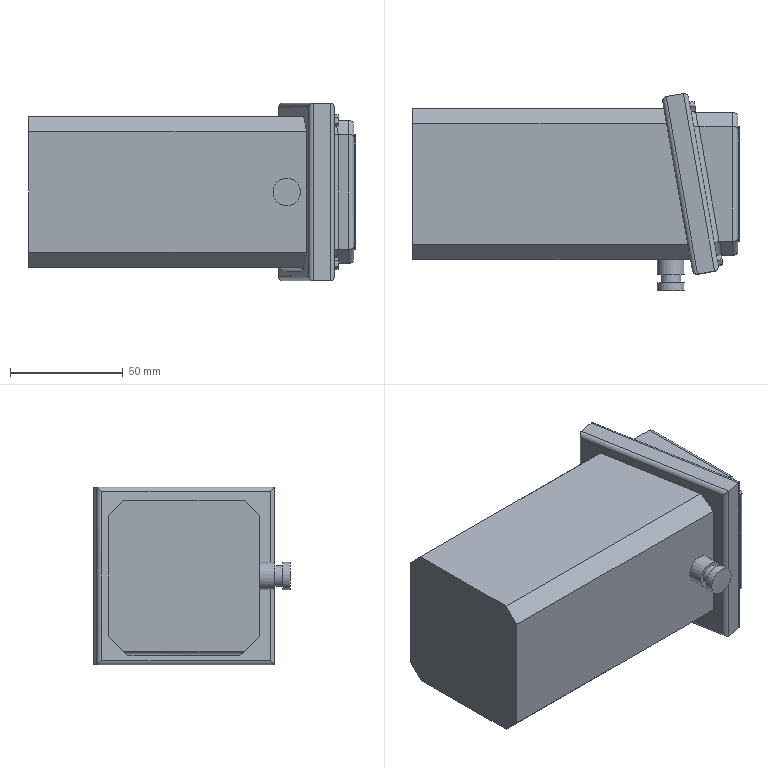Part | STEP file | Y2_JXH_80.step 5 | 1 solid | 173 faces | box 145 x 87.322 x 78.75 mm | volume 651359 mm3 | plane 108 | cylinder 65 | commonest cylinder face diameters 0.507 x16 4.548 x16 3.938 x9 2.791 x5 2.233 x4 3.908 x3